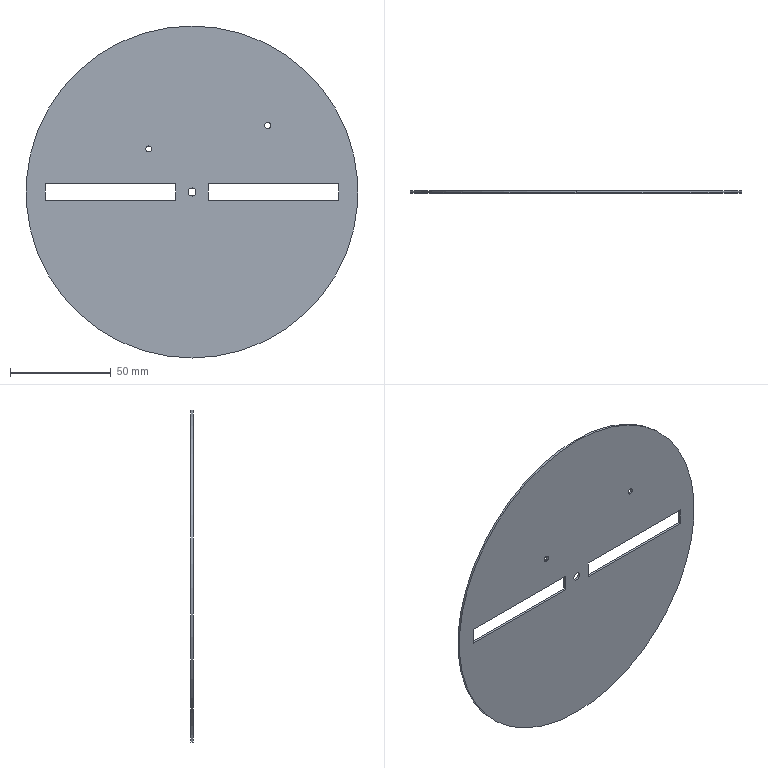Part | SolidWorks | features Extrusion 1 | 1 solid | 18 faces | box 165 x 1 x 165 mm | volume 20280 mm3 | plane 10 | cylinder 8 | commonest cylinder face diameters 3 x4 4 x2 165 x2
STEP:
#1=CARTESIAN_POINT('',(0.,1.,-2.));
#2=VERTEX_POINT('',#1);
#3=CARTESIAN_POINT('',(0.,1.,2.));
#4=VERTEX_POINT('',#3);
#5=CARTESIAN_POINT('',(0.,1.,0.));
#6=DIRECTION('',(0.,1.,0.));
#7=DIRECTION('',(0.,0.,1.));
#8=AXIS2_PLACEMENT_3D('',#5,#6,#7);
#9=CIRCLE('',#8,2.);
#10=EDGE_CURVE('',#2,#4,#9,.T.);
#11=ORIENTED_EDGE('',*,*,#10,.T.);
#12=CARTESIAN_POINT('',(0.,0.,2.));
#13=VERTEX_POINT('',#12);
#14=CARTESIAN_POINT('',(0.,1.,2.));
#15=DIRECTION('',(0.,-1.,0.));
#16=VECTOR('',#15,1000.);
#17=LINE('',#14,#16);
#18=EDGE_CURVE('',#4,#13,#17,.T.);
#19=ORIENTED_EDGE('',*,*,#18,.T.);
#20=CARTESIAN_POINT('',(0.,0.,-2.));
#21=VERTEX_POINT('',#20);
#22=CARTESIAN_POINT('',(0.,0.,0.));
#23=DIRECTION('',(0.,1.,0.));
#24=DIRECTION('',(0.,0.,1.));
#25=AXIS2_PLACEMENT_3D('',#22,#23,#24);
#26=CIRCLE('',#25,2.);
#27=EDGE_CURVE('',#21,#13,#26,.T.);
#28=ORIENTED_EDGE('',*,*,#27,.F.);
#29=CARTESIAN_POINT('',(0.,1.,-2.));
#30=DIRECTION('',(0.,-1.,0.));
#31=VECTOR('',#30,1000.);
#32=LINE('',#29,#31);
#33=EDGE_CURVE('',#2,#21,#32,.T.);
#34=ORIENTED_EDGE('',*,*,#33,.F.);
#35=EDGE_LOOP('',(#11,#19,#28,#34));
#36=FACE_OUTER_BOUND('',#35,.T.);
#37=CARTESIAN_POINT('',(0.,1.,0.));
#38=DIRECTION('',(0.,-1.,0.));
#39=DIRECTION('',(0.,0.,-1.));
#40=AXIS2_PLACEMENT_3D('',#37,#38,#39);
#41=CYLINDRICAL_SURFACE('',#40,2.);
#42=ADVANCED_FACE('',(#36),#41,.F.);
#43=CARTESIAN_POINT('',(37.6,1.,31.5));
#44=VERTEX_POINT('',#43);
#45=CARTESIAN_POINT('',(37.6,1.,34.5));
#46=VERTEX_POINT('',#45);
#47=CARTESIAN_POINT('',(37.6,1.,33.));
#48=DIRECTION('',(0.,1.,0.));
#49=DIRECTION('',(0.,0.,1.));
#50=AXIS2_PLACEMENT_3D('',#47,#48,#49);
#51=CIRCLE('',#50,1.5);
#52=EDGE_CURVE('',#44,#46,#51,.T.);
#53=ORIENTED_EDGE('',*,*,#52,.T.);
#54=CARTESIAN_POINT('',(37.6,0.,34.5));
#55=VERTEX_POINT('',#54);
#56=CARTESIAN_POINT('',(37.6,1.,34.5));
#57=DIRECTION('',(0.,-1.,0.));
#58=VECTOR('',#57,1000.);
#59=LINE('',#56,#58);
#60=EDGE_CURVE('',#46,#55,#59,.T.);
#61=ORIENTED_EDGE('',*,*,#60,.T.);
#62=CARTESIAN_POINT('',(37.6,0.,31.5));
#63=VERTEX_POINT('',#62);
#64=CARTESIAN_POINT('',(37.6,0.,33.));
#65=DIRECTION('',(0.,1.,0.));
#66=DIRECTION('',(0.,0.,1.));
#67=AXIS2_PLACEMENT_3D('',#64,#65,#66);
#68=CIRCLE('',#67,1.5);
#69=EDGE_CURVE('',#63,#55,#68,.T.);
#70=ORIENTED_EDGE('',*,*,#69,.F.);
#71=CARTESIAN_POINT('',(37.6,1.,31.5));
#72=DIRECTION('',(0.,-1.,0.));
#73=VECTOR('',#72,1000.);
#74=LINE('',#71,#73);
#75=EDGE_CURVE('',#44,#63,#74,.T.);
#76=ORIENTED_EDGE('',*,*,#75,.F.);
#77=EDGE_LOOP('',(#53,#61,#70,#76));
#78=FACE_OUTER_BOUND('',#77,.T.);
#79=CARTESIAN_POINT('',(37.6,1.,33.));
#80=DIRECTION('',(0.,-1.,0.));
#81=DIRECTION('',(0.,0.,-1.));
#82=AXIS2_PLACEMENT_3D('',#79,#80,#81);
#83=CYLINDRICAL_SURFACE('',#82,1.5);
#84=ADVANCED_FACE('',(#78),#83,.F.);
#85=CARTESIAN_POINT('',(-21.4,1.,19.9));
#86=VERTEX_POINT('',#85);
#87=CARTESIAN_POINT('',(-21.4,1.,22.9));
#88=VERTEX_POINT('',#87);
#89=CARTESIAN_POINT('',(-21.4,1.,21.4));
#90=DIRECTION('',(0.,1.,0.));
#91=DIRECTION('',(0.,0.,1.));
#92=AXIS2_PLACEMENT_3D('',#89,#90,#91);
#93=CIRCLE('',#92,1.5);
#94=EDGE_CURVE('',#86,#88,#93,.T.);
#95=ORIENTED_EDGE('',*,*,#94,.T.);
#96=CARTESIAN_POINT('',(-21.4,0.,22.9));
#97=VERTEX_POINT('',#96);
#98=CARTESIAN_POINT('',(-21.4,1.,22.9));
#99=DIRECTION('',(0.,-1.,0.));
#100=VECTOR('',#99,1000.);
#101=LINE('',#98,#100);
#102=EDGE_CURVE('',#88,#97,#101,.T.);
#103=ORIENTED_EDGE('',*,*,#102,.T.);
#104=CARTESIAN_POINT('',(-21.4,0.,19.9));
#105=VERTEX_POINT('',#104);
#106=CARTESIAN_POINT('',(-21.4,0.,21.4));
#107=DIRECTION('',(0.,1.,0.));
#108=DIRECTION('',(0.,0.,1.));
#109=AXIS2_PLACEMENT_3D('',#106,#107,#108);
#110=CIRCLE('',#109,1.5);
#111=EDGE_CURVE('',#105,#97,#110,.T.);
#112=ORIENTED_EDGE('',*,*,#111,.F.);
#113=CARTESIAN_POINT('',(-21.4,1.,19.9));
#114=DIRECTION('',(0.,-1.,0.));
#115=VECTOR('',#114,1000.);
#116=LINE('',#113,#115);
#117=EDGE_CURVE('',#86,#105,#116,.T.);
#118=ORIENTED_EDGE('',*,*,#117,.F.);
#119=EDGE_LOOP('',(#95,#103,#112,#118));
#120=FACE_OUTER_BOUND('',#119,.T.);
#121=CARTESIAN_POINT('',(-21.4,1.,21.4));
#122=DIRECTION('',(0.,-1.,0.));
#123=DIRECTION('',(0.,0.,-1.));
#124=AXIS2_PLACEMENT_3D('',#121,#122,#123);
#125=CYLINDRICAL_SURFACE('',#124,1.5);
#126=ADVANCED_FACE('',(#120),#125,.F.);
#127=CARTESIAN_POINT('',(0.,1.,82.5));
#128=VERTEX_POINT('',#127);
#129=CARTESIAN_POINT('',(0.,1.,-82.5));
#130=VERTEX_POINT('',#129);
#131=CARTESIAN_POINT('',(0.,1.,0.));
#132=DIRECTION('',(0.,1.,0.));
#133=DIRECTION('',(0.,0.,1.));
#134=AXIS2_PLACEMENT_3D('',#131,#132,#133);
#135=CIRCLE('',#134,82.5);
#136=EDGE_CURVE('',#128,#130,#135,.T.);
#137=ORIENTED_EDGE('',*,*,#136,.F.);
#138=CARTESIAN_POINT('',(0.,0.,82.5));
#139=VERTEX_POINT('',#138);
#140=CARTESIAN_POINT('',(0.,1.,82.5));
#141=DIRECTION('',(0.,-1.,0.));
#142=VECTOR('',#141,1000.);
#143=LINE('',#140,#142);
#144=EDGE_CURVE('',#128,#139,#143,.T.);
#145=ORIENTED_EDGE('',*,*,#144,.T.);
#146=CARTESIAN_POINT('',(0.,0.,-82.5));
#147=VERTEX_POINT('',#146);
#148=CARTESIAN_POINT('',(0.,0.,0.));
#149=DIRECTION('',(0.,1.,0.));
#150=DIRECTION('',(0.,0.,1.));
#151=AXIS2_PLACEMENT_3D('',#148,#149,#150);
#152=CIRCLE('',#151,82.5);
#153=EDGE_CURVE('',#139,#147,#152,.T.);
#154=ORIENTED_EDGE('',*,*,#153,.T.);
#155=CARTESIAN_POINT('',(0.,1.,-82.5));
#156=DIRECTION('',(0.,-1.,0.));
#157=VECTOR('',#156,1000.);
#158=LINE('',#155,#157);
#159=EDGE_CURVE('',#130,#147,#158,.T.);
#160=ORIENTED_EDGE('',*,*,#159,.F.);
#161=EDGE_LOOP('',(#137,#145,#154,#160));
#162=FACE_OUTER_BOUND('',#161,.T.);
#163=CARTESIAN_POINT('',(0.,1.,0.));
#164=DIRECTION('',(0.,-1.,0.));
#165=DIRECTION('',(0.,0.,-1.));
#166=AXIS2_PLACEMENT_3D('',#163,#164,#165);
#167=CYLINDRICAL_SURFACE('',#166,82.5);
#168=ADVANCED_FACE('',(#162),#167,.T.);
#169=ORIENTED_EDGE('',*,*,#52,.F.);
#170=CARTESIAN_POINT('',(37.6,1.,33.));
#171=DIRECTION('',(0.,1.,0.));
#172=DIRECTION('',(0.,0.,1.));
#173=AXIS2_PLACEMENT_3D('',#170,#171,#172);
#174=CIRCLE('',#173,1.5);
#175=EDGE_CURVE('',#46,#44,#174,.T.);
#176=ORIENTED_EDGE('',*,*,#175,.F.);
#177=EDGE_LOOP('',(#169,#176));
#178=FACE_BOUND('',#177,.T.);
#179=CARTESIAN_POINT('',(8.05,1.,-4.15));
#180=VERTEX_POINT('',#179);
#181=CARTESIAN_POINT('',(8.05,1.,4.15));
#182=VERTEX_POINT('',#181);
#183=CARTESIAN_POINT('',(8.05,1.,-4.15));
#184=DIRECTION('',(0.,0.,1.));
#185=VECTOR('',#184,1000.);
#186=LINE('',#183,#185);
#187=EDGE_CURVE('',#180,#182,#186,.T.);
#188=ORIENTED_EDGE('',*,*,#187,.F.);
#189=CARTESIAN_POINT('',(72.85,1.,-4.15));
#190=VERTEX_POINT('',#189);
#191=CARTESIAN_POINT('',(72.85,1.,-4.15));
#192=DIRECTION('',(-1.,0.,0.));
#193=VECTOR('',#192,1000.);
#194=LINE('',#191,#193);
#195=EDGE_CURVE('',#190,#180,#194,.T.);
#196=ORIENTED_EDGE('',*,*,#195,.F.);
#197=CARTESIAN_POINT('',(72.85,1.,4.15));
#198=VERTEX_POINT('',#197);
#199=CARTESIAN_POINT('',(72.85,1.,-4.15));
#200=DIRECTION('',(0.,0.,-1.));
#201=VECTOR('',#200,1000.);
#202=LINE('',#199,#201);
#203=EDGE_CURVE('',#198,#190,#202,.T.);
#204=ORIENTED_EDGE('',*,*,#203,.F.);
#205=CARTESIAN_POINT('',(72.85,1.,4.15));
#206=DIRECTION('',(1.,0.,0.));
#207=VECTOR('',#206,1000.);
#208=LINE('',#205,#207);
#209=EDGE_CURVE('',#182,#198,#208,.T.);
#210=ORIENTED_EDGE('',*,*,#209,.F.);
#211=EDGE_LOOP('',(#188,#196,#204,#210));
#212=FACE_BOUND('',#211,.T.);
#213=CARTESIAN_POINT('',(0.,1.,0.));
#214=DIRECTION('',(0.,1.,0.));
#215=DIRECTION('',(0.,0.,1.));
#216=AXIS2_PLACEMENT_3D('',#213,#214,#215);
#217=CIRCLE('',#216,82.5);
#218=EDGE_CURVE('',#130,#128,#217,.T.);
#219=ORIENTED_EDGE('',*,*,#218,.T.);
#220=ORIENTED_EDGE('',*,*,#136,.T.);
#221=EDGE_LOOP('',(#219,#220));
#222=FACE_OUTER_BOUND('',#221,.T.);
#223=CARTESIAN_POINT('',(-72.85,1.,4.15));
#224=VERTEX_POINT('',#223);
#225=CARTESIAN_POINT('',(-8.05,1.,4.15));
#226=VERTEX_POINT('',#225);
#227=CARTESIAN_POINT('',(-72.85,1.,4.15));
#228=DIRECTION('',(1.,0.,0.));
#229=VECTOR('',#228,1000.);
#230=LINE('',#227,#229);
#231=EDGE_CURVE('',#224,#226,#230,.T.);
#232=ORIENTED_EDGE('',*,*,#231,.F.);
#233=CARTESIAN_POINT('',(-72.85,1.,-4.15));
#234=VERTEX_POINT('',#233);
#235=CARTESIAN_POINT('',(-72.85,1.,-4.15));
#236=DIRECTION('',(0.,0.,1.));
#237=VECTOR('',#236,1000.);
#238=LINE('',#235,#237);
#239=EDGE_CURVE('',#234,#224,#238,.T.);
#240=ORIENTED_EDGE('',*,*,#239,.F.);
#241=CARTESIAN_POINT('',(-8.05,1.,-4.15));
#242=VERTEX_POINT('',#241);
#243=CARTESIAN_POINT('',(-72.85,1.,-4.15));
#244=DIRECTION('',(-1.,0.,0.));
#245=VECTOR('',#244,1000.);
#246=LINE('',#243,#245);
#247=EDGE_CURVE('',#242,#234,#246,.T.);
#248=ORIENTED_EDGE('',*,*,#247,.F.);
#249=CARTESIAN_POINT('',(-8.05,1.,-4.15));
#250=DIRECTION('',(0.,0.,-1.));
#251=VECTOR('',#250,1000.);
#252=LINE('',#249,#251);
#253=EDGE_CURVE('',#226,#242,#252,.T.);
#254=ORIENTED_EDGE('',*,*,#253,.F.);
#255=EDGE_LOOP('',(#232,#240,#248,#254));
#256=FACE_BOUND('',#255,.T.);
#257=ORIENTED_EDGE('',*,*,#94,.F.);
#258=CARTESIAN_POINT('',(-21.4,1.,21.4));
#259=DIRECTION('',(0.,1.,0.));
#260=DIRECTION('',(0.,0.,1.));
#261=AXIS2_PLACEMENT_3D('',#258,#259,#260);
#262=CIRCLE('',#261,1.5);
#263=EDGE_CURVE('',#88,#86,#262,.T.);
#264=ORIENTED_EDGE('',*,*,#263,.F.);
#265=EDGE_LOOP('',(#257,#264));
#266=FACE_BOUND('',#265,.T.);
#267=ORIENTED_EDGE('',*,*,#10,.F.);
#268=CARTESIAN_POINT('',(0.,1.,0.));
#269=DIRECTION('',(0.,1.,0.));
#270=DIRECTION('',(0.,0.,1.));
#271=AXIS2_PLACEMENT_3D('',#268,#269,#270);
#272=CIRCLE('',#271,2.);
#273=EDGE_CURVE('',#4,#2,#272,.T.);
#274=ORIENTED_EDGE('',*,*,#273,.F.);
#275=EDGE_LOOP('',(#267,#274));
#276=FACE_BOUND('',#275,.T.);
#277=CARTESIAN_POINT('',(0.,1.,0.));
#278=DIRECTION('',(0.,1.,0.));
#279=DIRECTION('',(0.,0.,1.));
#280=AXIS2_PLACEMENT_3D('',#277,#278,#279);
#281=PLANE('',#280);
#282=ADVANCED_FACE('',(#178,#212,#222,#256,#266,#276),#281,.T.);
#283=ORIENTED_EDGE('',*,*,#69,.T.);
#284=CARTESIAN_POINT('',(37.6,0.,33.));
#285=DIRECTION('',(0.,1.,0.));
#286=DIRECTION('',(0.,0.,1.));
#287=AXIS2_PLACEMENT_3D('',#284,#285,#286);
#288=CIRCLE('',#287,1.5);
#289=EDGE_CURVE('',#55,#63,#288,.T.);
#290=ORIENTED_EDGE('',*,*,#289,.T.);
#291=EDGE_LOOP('',(#283,#290));
#292=FACE_BOUND('',#291,.T.);
#293=CARTESIAN_POINT('',(72.85,0.,-4.15));
#294=VERTEX_POINT('',#293);
#295=CARTESIAN_POINT('',(8.05,0.,-4.15));
#296=VERTEX_POINT('',#295);
#297=CARTESIAN_POINT('',(72.85,0.,-4.15));
#298=DIRECTION('',(-1.,0.,0.));
#299=VECTOR('',#298,1000.);
#300=LINE('',#297,#299);
#301=EDGE_CURVE('',#294,#296,#300,.T.);
#302=ORIENTED_EDGE('',*,*,#301,.T.);
#303=CARTESIAN_POINT('',(8.05,0.,4.15));
#304=VERTEX_POINT('',#303);
#305=CARTESIAN_POINT('',(8.05,0.,-4.15));
#306=DIRECTION('',(0.,0.,1.));
#307=VECTOR('',#306,1000.);
#308=LINE('',#305,#307);
#309=EDGE_CURVE('',#296,#304,#308,.T.);
#310=ORIENTED_EDGE('',*,*,#309,.T.);
#311=CARTESIAN_POINT('',(72.85,0.,4.15));
#312=VERTEX_POINT('',#311);
#313=CARTESIAN_POINT('',(72.85,0.,4.15));
#314=DIRECTION('',(1.,0.,0.));
#315=VECTOR('',#314,1000.);
#316=LINE('',#313,#315);
#317=EDGE_CURVE('',#304,#312,#316,.T.);
#318=ORIENTED_EDGE('',*,*,#317,.T.);
#319=CARTESIAN_POINT('',(72.85,0.,-4.15));
#320=DIRECTION('',(0.,0.,-1.));
#321=VECTOR('',#320,1000.);
#322=LINE('',#319,#321);
#323=EDGE_CURVE('',#312,#294,#322,.T.);
#324=ORIENTED_EDGE('',*,*,#323,.T.);
#325=EDGE_LOOP('',(#302,#310,#318,#324));
#326=FACE_BOUND('',#325,.T.);
#327=CARTESIAN_POINT('',(0.,0.,0.));
#328=DIRECTION('',(0.,1.,0.));
#329=DIRECTION('',(0.,0.,1.));
#330=AXIS2_PLACEMENT_3D('',#327,#328,#329);
#331=CIRCLE('',#330,82.5);
#332=EDGE_CURVE('',#147,#139,#331,.T.);
#333=ORIENTED_EDGE('',*,*,#332,.F.);
#334=ORIENTED_EDGE('',*,*,#153,.F.);
#335=EDGE_LOOP('',(#333,#334));
#336=FACE_OUTER_BOUND('',#335,.T.);
#337=CARTESIAN_POINT('',(-72.85,0.,-4.15));
#338=VERTEX_POINT('',#337);
#339=CARTESIAN_POINT('',(-72.85,0.,4.15));
#340=VERTEX_POINT('',#339);
#341=CARTESIAN_POINT('',(-72.85,0.,-4.15));
#342=DIRECTION('',(0.,0.,1.));
#343=VECTOR('',#342,1000.);
#344=LINE('',#341,#343);
#345=EDGE_CURVE('',#338,#340,#344,.T.);
#346=ORIENTED_EDGE('',*,*,#345,.T.);
#347=CARTESIAN_POINT('',(-8.05,0.,4.15));
#348=VERTEX_POINT('',#347);
#349=CARTESIAN_POINT('',(-72.85,0.,4.15));
#350=DIRECTION('',(1.,0.,0.));
#351=VECTOR('',#350,1000.);
#352=LINE('',#349,#351);
#353=EDGE_CURVE('',#340,#348,#352,.T.);
#354=ORIENTED_EDGE('',*,*,#353,.T.);
#355=CARTESIAN_POINT('',(-8.05,0.,-4.15));
#356=VERTEX_POINT('',#355);
#357=CARTESIAN_POINT('',(-8.05,0.,-4.15));
#358=DIRECTION('',(0.,0.,-1.));
#359=VECTOR('',#358,1000.);
#360=LINE('',#357,#359);
#361=EDGE_CURVE('',#348,#356,#360,.T.);
#362=ORIENTED_EDGE('',*,*,#361,.T.);
#363=CARTESIAN_POINT('',(-72.85,0.,-4.15));
#364=DIRECTION('',(-1.,0.,0.));
#365=VECTOR('',#364,1000.);
#366=LINE('',#363,#365);
#367=EDGE_CURVE('',#356,#338,#366,.T.);
#368=ORIENTED_EDGE('',*,*,#367,.T.);
#369=EDGE_LOOP('',(#346,#354,#362,#368));
#370=FACE_BOUND('',#369,.T.);
#371=ORIENTED_EDGE('',*,*,#111,.T.);
#372=CARTESIAN_POINT('',(-21.4,0.,21.4));
#373=DIRECTION('',(0.,1.,0.));
#374=DIRECTION('',(0.,0.,1.));
#375=AXIS2_PLACEMENT_3D('',#372,#373,#374);
#376=CIRCLE('',#375,1.5);
#377=EDGE_CURVE('',#97,#105,#376,.T.);
#378=ORIENTED_EDGE('',*,*,#377,.T.);
#379=EDGE_LOOP('',(#371,#378));
#380=FACE_BOUND('',#379,.T.);
#381=ORIENTED_EDGE('',*,*,#27,.T.);
#382=CARTESIAN_POINT('',(0.,0.,0.));
#383=DIRECTION('',(0.,1.,0.));
#384=DIRECTION('',(0.,0.,1.));
#385=AXIS2_PLACEMENT_3D('',#382,#383,#384);
#386=CIRCLE('',#385,2.);
#387=EDGE_CURVE('',#13,#21,#386,.T.);
#388=ORIENTED_EDGE('',*,*,#387,.T.);
#389=EDGE_LOOP('',(#381,#388));
#390=FACE_BOUND('',#389,.T.);
#391=CARTESIAN_POINT('',(0.,0.,0.));
#392=DIRECTION('',(0.,1.,0.));
#393=DIRECTION('',(0.,0.,1.));
#394=AXIS2_PLACEMENT_3D('',#391,#392,#393);
#395=PLANE('',#394);
#396=ADVANCED_FACE('',(#292,#326,#336,#370,#380,#390),#395,.F.);
#397=ORIENTED_EDGE('',*,*,#144,.F.);
#398=ORIENTED_EDGE('',*,*,#218,.F.);
#399=ORIENTED_EDGE('',*,*,#159,.T.);
#400=ORIENTED_EDGE('',*,*,#332,.T.);
#401=EDGE_LOOP('',(#397,#398,#399,#400));
#402=FACE_OUTER_BOUND('',#401,.T.);
#403=CARTESIAN_POINT('',(0.,1.,0.));
#404=DIRECTION('',(0.,-1.,0.));
#405=DIRECTION('',(0.,0.,-1.));
#406=AXIS2_PLACEMENT_3D('',#403,#404,#405);
#407=CYLINDRICAL_SURFACE('',#406,82.5);
#408=ADVANCED_FACE('',(#402),#407,.T.);
#409=ORIENTED_EDGE('',*,*,#345,.F.);
#410=CARTESIAN_POINT('',(-72.85,1.,-4.15));
#411=DIRECTION('',(0.,-1.,0.));
#412=VECTOR('',#411,1000.);
#413=LINE('',#410,#412);
#414=EDGE_CURVE('',#234,#338,#413,.T.);
#415=ORIENTED_EDGE('',*,*,#414,.F.);
#416=ORIENTED_EDGE('',*,*,#239,.T.);
#417=CARTESIAN_POINT('',(-72.85,1.,4.15));
#418=DIRECTION('',(0.,-1.,0.));
#419=VECTOR('',#418,1000.);
#420=LINE('',#417,#419);
#421=EDGE_CURVE('',#224,#340,#420,.T.);
#422=ORIENTED_EDGE('',*,*,#421,.T.);
#423=EDGE_LOOP('',(#409,#415,#416,#422));
#424=FACE_OUTER_BOUND('',#423,.T.);
#425=CARTESIAN_POINT('',(-72.85,1.,-4.15));
#426=DIRECTION('',(1.,0.,0.));
#427=DIRECTION('',(0.,0.,-1.));
#428=AXIS2_PLACEMENT_3D('',#425,#426,#427);
#429=PLANE('',#428);
#430=ADVANCED_FACE('',(#424),#429,.T.);
#431=ORIENTED_EDGE('',*,*,#353,.F.);
#432=ORIENTED_EDGE('',*,*,#421,.F.);
#433=ORIENTED_EDGE('',*,*,#231,.T.);
#434=CARTESIAN_POINT('',(-8.05,1.,4.15));
#435=DIRECTION('',(0.,-1.,0.));
#436=VECTOR('',#435,1000.);
#437=LINE('',#434,#436);
#438=EDGE_CURVE('',#226,#348,#437,.T.);
#439=ORIENTED_EDGE('',*,*,#438,.T.);
#440=EDGE_LOOP('',(#431,#432,#433,#439));
#441=FACE_OUTER_BOUND('',#440,.T.);
#442=CARTESIAN_POINT('',(-72.85,1.,4.15));
#443=DIRECTION('',(0.,0.,-1.));
#444=DIRECTION('',(-1.,0.,0.));
#445=AXIS2_PLACEMENT_3D('',#442,#443,#444);
#446=PLANE('',#445);
#447=ADVANCED_FACE('',(#441),#446,.T.);
#448=ORIENTED_EDGE('',*,*,#361,.F.);
#449=ORIENTED_EDGE('',*,*,#438,.F.);
#450=ORIENTED_EDGE('',*,*,#253,.T.);
#451=CARTESIAN_POINT('',(-8.05,1.,-4.15));
#452=DIRECTION('',(0.,-1.,0.));
#453=VECTOR('',#452,1000.);
#454=LINE('',#451,#453);
#455=EDGE_CURVE('',#242,#356,#454,.T.);
#456=ORIENTED_EDGE('',*,*,#455,.T.);
#457=EDGE_LOOP('',(#448,#449,#450,#456));
#458=FACE_OUTER_BOUND('',#457,.T.);
#459=CARTESIAN_POINT('',(-8.05,1.,-4.15));
#460=DIRECTION('',(-1.,0.,0.));
#461=DIRECTION('',(0.,0.,1.));
#462=AXIS2_PLACEMENT_3D('',#459,#460,#461);
#463=PLANE('',#462);
#464=ADVANCED_FACE('',(#458),#463,.T.);
#465=ORIENTED_EDGE('',*,*,#367,.F.);
#466=ORIENTED_EDGE('',*,*,#455,.F.);
#467=ORIENTED_EDGE('',*,*,#247,.T.);
#468=ORIENTED_EDGE('',*,*,#414,.T.);
#469=EDGE_LOOP('',(#465,#466,#467,#468));
#470=FACE_OUTER_BOUND('',#469,.T.);
#471=CARTESIAN_POINT('',(-72.85,1.,-4.15));
#472=DIRECTION('',(0.,0.,1.));
#473=DIRECTION('',(1.,0.,0.));
#474=AXIS2_PLACEMENT_3D('',#471,#472,#473);
#475=PLANE('',#474);
#476=ADVANCED_FACE('',(#470),#475,.T.);
#477=ORIENTED_EDGE('',*,*,#301,.F.);
#478=CARTESIAN_POINT('',(72.85,1.,-4.15));
#479=DIRECTION('',(0.,-1.,0.));
#480=VECTOR('',#479,1000.);
#481=LINE('',#478,#480);
#482=EDGE_CURVE('',#190,#294,#481,.T.);
#483=ORIENTED_EDGE('',*,*,#482,.F.);
#484=ORIENTED_EDGE('',*,*,#195,.T.);
#485=CARTESIAN_POINT('',(8.05,1.,-4.15));
#486=DIRECTION('',(0.,-1.,0.));
#487=VECTOR('',#486,1000.);
#488=LINE('',#485,#487);
#489=EDGE_CURVE('',#180,#296,#488,.T.);
#490=ORIENTED_EDGE('',*,*,#489,.T.);
#491=EDGE_LOOP('',(#477,#483,#484,#490));
#492=FACE_OUTER_BOUND('',#491,.T.);
#493=CARTESIAN_POINT('',(72.85,1.,-4.15));
#494=DIRECTION('',(0.,0.,1.));
#495=DIRECTION('',(1.,0.,0.));
#496=AXIS2_PLACEMENT_3D('',#493,#494,#495);
#497=PLANE('',#496);
#498=ADVANCED_FACE('',(#492),#497,.T.);
#499=ORIENTED_EDGE('',*,*,#309,.F.);
#500=ORIENTED_EDGE('',*,*,#489,.F.);
#501=ORIENTED_EDGE('',*,*,#187,.T.);
#502=CARTESIAN_POINT('',(8.05,1.,4.15));
#503=DIRECTION('',(0.,-1.,0.));
#504=VECTOR('',#503,1000.);
#505=LINE('',#502,#504);
#506=EDGE_CURVE('',#182,#304,#505,.T.);
#507=ORIENTED_EDGE('',*,*,#506,.T.);
#508=EDGE_LOOP('',(#499,#500,#501,#507));
#509=FACE_OUTER_BOUND('',#508,.T.);
#510=CARTESIAN_POINT('',(8.05,1.,-4.15));
#511=DIRECTION('',(1.,0.,0.));
#512=DIRECTION('',(0.,0.,-1.));
#513=AXIS2_PLACEMENT_3D('',#510,#511,#512);
#514=PLANE('',#513);
#515=ADVANCED_FACE('',(#509),#514,.T.);
#516=ORIENTED_EDGE('',*,*,#317,.F.);
#517=ORIENTED_EDGE('',*,*,#506,.F.);
#518=ORIENTED_EDGE('',*,*,#209,.T.);
#519=CARTESIAN_POINT('',(72.85,1.,4.15));
#520=DIRECTION('',(0.,-1.,0.));
#521=VECTOR('',#520,1000.);
#522=LINE('',#519,#521);
#523=EDGE_CURVE('',#198,#312,#522,.T.);
#524=ORIENTED_EDGE('',*,*,#523,.T.);
#525=EDGE_LOOP('',(#516,#517,#518,#524));
#526=FACE_OUTER_BOUND('',#525,.T.);
#527=CARTESIAN_POINT('',(72.85,1.,4.15));
#528=DIRECTION('',(0.,0.,-1.));
#529=DIRECTION('',(-1.,0.,0.));
#530=AXIS2_PLACEMENT_3D('',#527,#528,#529);
#531=PLANE('',#530);
#532=ADVANCED_FACE('',(#526),#531,.T.);
#533=ORIENTED_EDGE('',*,*,#323,.F.);
#534=ORIENTED_EDGE('',*,*,#523,.F.);
#535=ORIENTED_EDGE('',*,*,#203,.T.);
#536=ORIENTED_EDGE('',*,*,#482,.T.);
#537=EDGE_LOOP('',(#533,#534,#535,#536));
#538=FACE_OUTER_BOUND('',#537,.T.);
#539=CARTESIAN_POINT('',(72.85,1.,-4.15));
#540=DIRECTION('',(-1.,0.,0.));
#541=DIRECTION('',(0.,0.,1.));
#542=AXIS2_PLACEMENT_3D('',#539,#540,#541);
#543=PLANE('',#542);
#544=ADVANCED_FACE('',(#538),#543,.T.);
#545=ORIENTED_EDGE('',*,*,#102,.F.);
#546=ORIENTED_EDGE('',*,*,#263,.T.);
#547=ORIENTED_EDGE('',*,*,#117,.T.);
#548=ORIENTED_EDGE('',*,*,#377,.F.);
#549=EDGE_LOOP('',(#545,#546,#547,#548));
#550=FACE_OUTER_BOUND('',#549,.T.);
#551=CARTESIAN_POINT('',(-21.4,1.,21.4));
#552=DIRECTION('',(0.,-1.,0.));
#553=DIRECTION('',(0.,0.,-1.));
#554=AXIS2_PLACEMENT_3D('',#551,#552,#553);
#555=CYLINDRICAL_SURFACE('',#554,1.5);
#556=ADVANCED_FACE('',(#550),#555,.F.);
#557=ORIENTED_EDGE('',*,*,#60,.F.);
#558=ORIENTED_EDGE('',*,*,#175,.T.);
#559=ORIENTED_EDGE('',*,*,#75,.T.);
#560=ORIENTED_EDGE('',*,*,#289,.F.);
#561=EDGE_LOOP('',(#557,#558,#559,#560));
#562=FACE_OUTER_BOUND('',#561,.T.);
#563=CARTESIAN_POINT('',(37.6,1.,33.));
#564=DIRECTION('',(0.,-1.,0.));
#565=DIRECTION('',(0.,0.,-1.));
#566=AXIS2_PLACEMENT_3D('',#563,#564,#565);
#567=CYLINDRICAL_SURFACE('',#566,1.5);
#568=ADVANCED_FACE('',(#562),#567,.F.);
#569=ORIENTED_EDGE('',*,*,#18,.F.);
#570=ORIENTED_EDGE('',*,*,#273,.T.);
#571=ORIENTED_EDGE('',*,*,#33,.T.);
#572=ORIENTED_EDGE('',*,*,#387,.F.);
#573=EDGE_LOOP('',(#569,#570,#571,#572));
#574=FACE_OUTER_BOUND('',#573,.T.);
#575=CARTESIAN_POINT('',(0.,1.,0.));
#576=DIRECTION('',(0.,-1.,0.));
#577=DIRECTION('',(0.,0.,-1.));
#578=AXIS2_PLACEMENT_3D('',#575,#576,#577);
#579=CYLINDRICAL_SURFACE('',#578,2.);
#580=ADVANCED_FACE('',(#574),#579,.F.);
#581=CLOSED_SHELL('',(#42,#84,#126,#168,#282,#396,#408,#430,#447,#464,#476,#498,#515,#532,#544,#556,#568,#580));
#582=MANIFOLD_SOLID_BREP('',#581);
#583=CARTESIAN_POINT('',(0.,0.,0.));
#584=DIRECTION('',(0.,0.,1.));
#585=DIRECTION('',(1.,0.,0.));
#586=AXIS2_PLACEMENT_3D('',#583,#584,#585);
#587=(LENGTH_UNIT()NAMED_UNIT(*)SI_UNIT(.MILLI.,.METRE.));
#588=UNCERTAINTY_MEASURE_WITH_UNIT(LENGTH_MEASURE(0.00001),#587,'','');
#589=(NAMED_UNIT(*)PLANE_ANGLE_UNIT()SI_UNIT($,.RADIAN.));
#590=(NAMED_UNIT(*)SI_UNIT($,.STERADIAN.)SOLID_ANGLE_UNIT());
#591=(GEOMETRIC_REPRESENTATION_CONTEXT(3)GLOBAL_UNCERTAINTY_ASSIGNED_CONTEXT((#588))GLOBAL_UNIT_ASSIGNED_CONTEXT((#587,#589,#590))REPRESENTATION_CONTEXT('',''));
#592=ADVANCED_BREP_SHAPE_REPRESENTATION('',(#582,#586),#591);